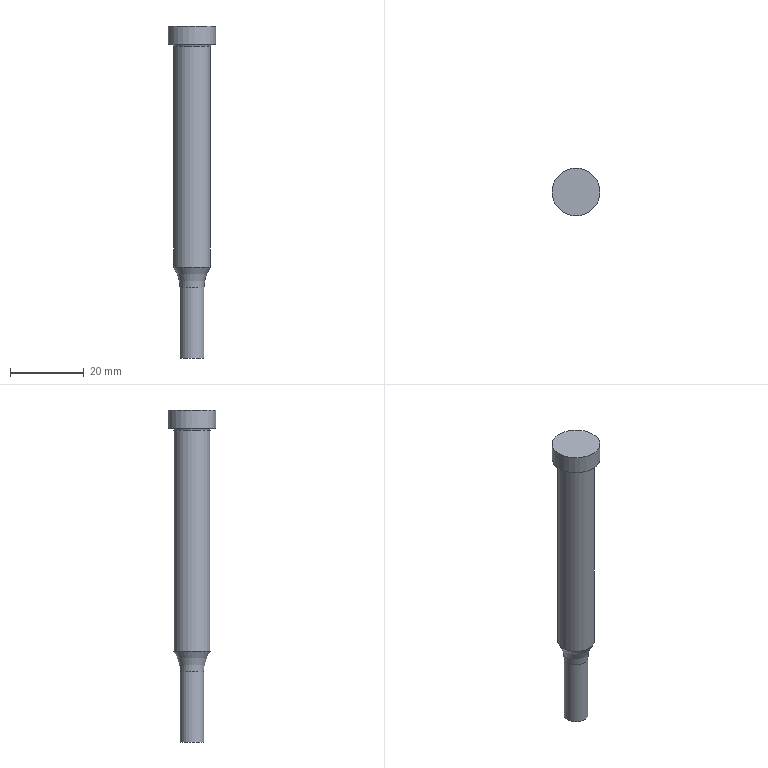Part | NX | features solid 2 | 1 solid | 8 faces | box 13 x 13 x 90 mm | volume 6298 mm3 | plane 3 | cylinder 3 | torus 2 | commonest cylinder face diameters 6.5 x1 10 x1 13 x1
STEP:
#1=CARTESIAN_POINT('',(105.5,-266.12,31.));
#2=VERTEX_POINT('',#1);
#3=CARTESIAN_POINT('',(100.,-266.12,31.));
#4=DIRECTION('',(0.,0.,1.));
#5=DIRECTION('',(1.,0.,0.));
#6=AXIS2_PLACEMENT_3D('',#3,#4,#5);
#7=CIRCLE('',#6,5.5);
#8=EDGE_CURVE('',#2,#2,#7,.F.);
#9=ORIENTED_EDGE('',*,*,#8,.F.);
#10=EDGE_LOOP('',(#9));
#11=FACE_BOUND('',#10,.T.);
#12=CARTESIAN_POINT('',(106.5,-266.12,31.));
#13=VERTEX_POINT('',#12);
#14=CARTESIAN_POINT('',(100.,-266.12,31.));
#15=DIRECTION('',(0.,0.,1.));
#16=DIRECTION('',(1.,0.,0.));
#17=AXIS2_PLACEMENT_3D('',#14,#15,#16);
#18=CIRCLE('',#17,6.5);
#19=EDGE_CURVE('',#13,#13,#18,.T.);
#20=ORIENTED_EDGE('',*,*,#19,.F.);
#21=EDGE_LOOP('',(#20));
#22=FACE_BOUND('',#21,.T.);
#23=CARTESIAN_POINT('',(100.,-266.12,31.));
#24=DIRECTION('',(0.,0.,-1.));
#25=DIRECTION('',(1.,0.,0.));
#26=AXIS2_PLACEMENT_3D('',#23,#24,#25);
#27=PLANE('',#26);
#28=ADVANCED_FACE('',(#11,#22),#27,.T.);
#29=ORIENTED_EDGE('',*,*,#19,.T.);
#30=EDGE_LOOP('',(#29));
#31=FACE_BOUND('',#30,.T.);
#32=CARTESIAN_POINT('',(106.5,-266.12,36.));
#33=VERTEX_POINT('',#32);
#34=CARTESIAN_POINT('',(100.,-266.12,36.));
#35=DIRECTION('',(0.,0.,1.));
#36=DIRECTION('',(1.,0.,0.));
#37=AXIS2_PLACEMENT_3D('',#34,#35,#36);
#38=CIRCLE('',#37,6.5);
#39=EDGE_CURVE('',#33,#33,#38,.T.);
#40=ORIENTED_EDGE('',*,*,#39,.F.);
#41=EDGE_LOOP('',(#40));
#42=FACE_BOUND('',#41,.T.);
#43=CARTESIAN_POINT('',(100.,-266.12,31.));
#44=DIRECTION('',(0.,0.,1.));
#45=DIRECTION('',(-1.,0.,0.));
#46=AXIS2_PLACEMENT_3D('',#43,#44,#45);
#47=CYLINDRICAL_SURFACE('',#46,6.5);
#48=ADVANCED_FACE('',(#31,#42),#47,.T.);
#49=ORIENTED_EDGE('',*,*,#39,.T.);
#50=EDGE_LOOP('',(#49));
#51=FACE_BOUND('',#50,.T.);
#52=CARTESIAN_POINT('',(100.,-266.12,36.));
#53=DIRECTION('',(0.,0.,-1.));
#54=DIRECTION('',(1.,0.,0.));
#55=AXIS2_PLACEMENT_3D('',#52,#53,#54);
#56=PLANE('',#55);
#57=ADVANCED_FACE('',(#51),#56,.F.);
#58=CARTESIAN_POINT('',(105.,-266.12,30.5));
#59=VERTEX_POINT('',#58);
#60=CARTESIAN_POINT('',(100.,-266.12,30.5));
#61=DIRECTION('',(0.,0.,1.));
#62=DIRECTION('',(1.,0.,0.));
#63=AXIS2_PLACEMENT_3D('',#60,#61,#62);
#64=CIRCLE('',#63,5.);
#65=EDGE_CURVE('',#59,#59,#64,.T.);
#66=ORIENTED_EDGE('',*,*,#65,.F.);
#67=EDGE_LOOP('',(#66));
#68=FACE_BOUND('',#67,.T.);
#69=CARTESIAN_POINT('',(105.,-266.12,-29.349));
#70=VERTEX_POINT('',#69);
#71=CARTESIAN_POINT('',(100.,-266.12,-29.349));
#72=DIRECTION('',(0.,0.,1.));
#73=DIRECTION('',(1.,0.,0.));
#74=AXIS2_PLACEMENT_3D('',#71,#72,#73);
#75=CIRCLE('',#74,5.);
#76=EDGE_CURVE('',#70,#70,#75,.T.);
#77=ORIENTED_EDGE('',*,*,#76,.T.);
#78=EDGE_LOOP('',(#77));
#79=FACE_BOUND('',#78,.T.);
#80=CARTESIAN_POINT('',(100.,-266.12,-29.349));
#81=DIRECTION('',(0.,0.,1.));
#82=DIRECTION('',(-1.,0.,0.));
#83=AXIS2_PLACEMENT_3D('',#80,#81,#82);
#84=CYLINDRICAL_SURFACE('',#83,5.);
#85=ADVANCED_FACE('',(#68,#79),#84,.T.);
#86=CARTESIAN_POINT('',(96.75,-266.12,-35.));
#87=VERTEX_POINT('',#86);
#88=CARTESIAN_POINT('',(100.,-266.12,-35.));
#89=DIRECTION('',(0.,0.,-1.));
#90=DIRECTION('',(-1.,0.,0.));
#91=AXIS2_PLACEMENT_3D('',#88,#89,#90);
#92=CIRCLE('',#91,3.25);
#93=EDGE_CURVE('',#87,#87,#92,.F.);
#94=ORIENTED_EDGE('',*,*,#93,.F.);
#95=EDGE_LOOP('',(#94));
#96=FACE_BOUND('',#95,.T.);
#97=CARTESIAN_POINT('',(103.25,-266.12,-54.));
#98=VERTEX_POINT('',#97);
#99=CARTESIAN_POINT('',(100.,-266.12,-54.));
#100=DIRECTION('',(0.,0.,1.));
#101=DIRECTION('',(1.,0.,0.));
#102=AXIS2_PLACEMENT_3D('',#99,#100,#101);
#103=CIRCLE('',#102,3.25);
#104=EDGE_CURVE('',#98,#98,#103,.T.);
#105=ORIENTED_EDGE('',*,*,#104,.T.);
#106=EDGE_LOOP('',(#105));
#107=FACE_BOUND('',#106,.T.);
#108=CARTESIAN_POINT('',(100.,-266.12,-54.));
#109=DIRECTION('',(0.,0.,1.));
#110=DIRECTION('',(-1.,0.,0.));
#111=AXIS2_PLACEMENT_3D('',#108,#109,#110);
#112=CYLINDRICAL_SURFACE('',#111,3.25);
#113=ADVANCED_FACE('',(#96,#107),#112,.T.);
#114=ORIENTED_EDGE('',*,*,#104,.F.);
#115=EDGE_LOOP('',(#114));
#116=FACE_BOUND('',#115,.T.);
#117=CARTESIAN_POINT('',(100.,-266.12,-54.));
#118=DIRECTION('',(0.,0.,-1.));
#119=DIRECTION('',(1.,0.,0.));
#120=AXIS2_PLACEMENT_3D('',#117,#118,#119);
#121=PLANE('',#120);
#122=ADVANCED_FACE('',(#116),#121,.T.);
#123=ORIENTED_EDGE('',*,*,#65,.T.);
#124=EDGE_LOOP('',(#123));
#125=FACE_BOUND('',#124,.T.);
#126=ORIENTED_EDGE('',*,*,#8,.T.);
#127=EDGE_LOOP('',(#126));
#128=FACE_BOUND('',#127,.T.);
#129=CARTESIAN_POINT('',(100.,-266.12,30.5));
#130=DIRECTION('',(0.,0.,-1.));
#131=DIRECTION('',(1.,0.,0.));
#132=AXIS2_PLACEMENT_3D('',#129,#130,#131);
#133=TOROIDAL_SURFACE('',#132,5.5,0.5);
#134=ADVANCED_FACE('',(#125,#128),#133,.F.);
#135=ORIENTED_EDGE('',*,*,#93,.T.);
#136=EDGE_LOOP('',(#135));
#137=FACE_BOUND('',#136,.T.);
#138=ORIENTED_EDGE('',*,*,#76,.F.);
#139=EDGE_LOOP('',(#138));
#140=FACE_BOUND('',#139,.T.);
#141=CARTESIAN_POINT('',(100.,-266.12,-35.));
#142=DIRECTION('',(0.,0.,1.));
#143=DIRECTION('',(-1.,0.,0.));
#144=AXIS2_PLACEMENT_3D('',#141,#142,#143);
#145=TOROIDAL_SURFACE('',#144,13.25,10.);
#146=ADVANCED_FACE('',(#137,#140),#145,.F.);
#147=CLOSED_SHELL('',(#28,#48,#57,#85,#113,#122,#134,#146));
#148=MANIFOLD_SOLID_BREP('',#147);
#149=(LENGTH_UNIT()NAMED_UNIT(*)SI_UNIT(.MILLI.,.METRE.));
#150=UNCERTAINTY_MEASURE_WITH_UNIT(LENGTH_MEASURE(0.00001),#149,'','');
#151=(NAMED_UNIT(*)PLANE_ANGLE_UNIT()SI_UNIT($,.RADIAN.));
#152=(NAMED_UNIT(*)SI_UNIT($,.STERADIAN.)SOLID_ANGLE_UNIT());
#153=(GEOMETRIC_REPRESENTATION_CONTEXT(3)GLOBAL_UNCERTAINTY_ASSIGNED_CONTEXT((#150))GLOBAL_UNIT_ASSIGNED_CONTEXT((#149,#151,#152))REPRESENTATION_CONTEXT('',''));
#154=ADVANCED_BREP_SHAPE_REPRESENTATION('',(#148),#153);